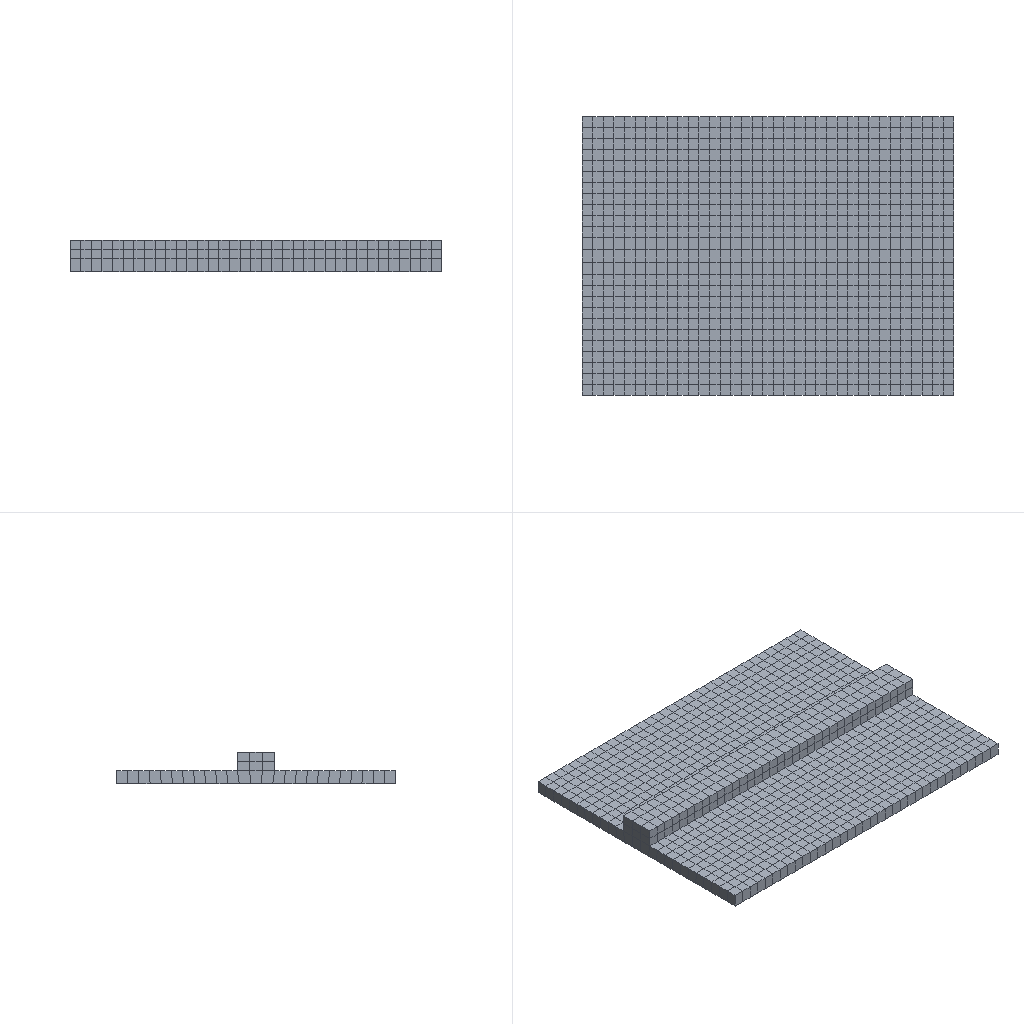Simulation study | abaqus
Set-up summary:
category,name,step,type,value,unit,region
solver,abaqus
solver,version,,,Abaqus/Standard 3DEXPERIENCE R2017x
solver,version,,,Abaqus/Standard 3DEXPERIENCE R2017x
units,not stated in the deck,,not stated
analysis,deck1,,static,coupled temperature-displacement; static
load_step,Step-del-all,Step-del-all,static,nlgeom=True
load_step,Step-add-1,Step-add-1,coupled temperature-displacement,nlgeom=True
load_step,Step-add-2,Step-add-2,coupled temperature-displacement,nlgeom=True
load_step,Step-add-3,Step-add-3,coupled temperature-displacement,nlgeom=True
load_step,Step-add-4,Step-add-4,coupled temperature-displacement,nlgeom=True
load_step,Step-add-5,Step-add-5,coupled temperature-displacement,nlgeom=True
load_step,Step-stop,Step-stop,coupled temperature-displacement,nlgeom=True
load_step,Step-add-6,Step-add-6,coupled temperature-displacement,nlgeom=True
load_step,Step-add-7,Step-add-7,coupled temperature-displacement,nlgeom=True
load_step,Step-add-8,Step-add-8,coupled temperature-displacement,nlgeom=True
load_step,Step-add-9,Step-add-9,coupled temperature-displacement,nlgeom=True
load_step,Step-add-10,Step-add-10,coupled temperature-displacement,nlgeom=True
load_step,Step-stop2,Step-stop2,coupled temperature-displacement,nlgeom=True
contact,interactions,,,general=0 pairs=0 ties=0
load_step,requested,,,13
mesh,nodes,,,2160
mesh,elements,,,1085
element_type,C3D8T,,solid,1085
load,load commands in deck,,count,1
bc,support commands in deck,,count,1
analysis,deck2,,static,coupled temperature-displacement; static
load_step,Step-del-all,Step-del-all,static,nlgeom=True
load_step,Step-add-1,Step-add-1,coupled temperature-displacement,nlgeom=True
load_step,Step-add-2,Step-add-2,coupled temperature-displacement,nlgeom=True
load_step,Step-add-3,Step-add-3,coupled temperature-displacement,nlgeom=True
load_step,Step-add-4,Step-add-4,coupled temperature-displacement,nlgeom=True
load_step,Step-add-5,Step-add-5,coupled temperature-displacement,nlgeom=True
load_step,Step-stop,Step-stop,coupled temperature-displacement,nlgeom=True
load_step,Step-add-6,Step-add-6,coupled temperature-displacement,nlgeom=True
load_step,Step-add-7,Step-add-7,coupled temperature-displacement,nlgeom=True
load_step,Step-add-8,Step-add-8,coupled temperature-displacement,nlgeom=True
load_step,Step-add-9,Step-add-9,coupled temperature-displacement,nlgeom=True
load_step,Step-add-10,Step-add-10,coupled temperature-displacement,nlgeom=True
load_step,Step-stop2,Step-stop2,coupled temperature-displacement,nlgeom=True
contact,interactions,,,general=0 pairs=0 ties=0
load_step,requested,,,13
mesh,nodes,,,2160
mesh,elements,,,1085
element_type,C3D8T,,solid,1085
load,load commands in deck,,count,1
bc,support commands in deck,,count,1
material,INCONEL,,in results
material,STEEL,,in results
material,INCONEL,,in results
material,STEEL,,in results
check,setup vs results,,match,"per instance, exact: element labels, types and connectivity; labels of the nodes the elements use; coordinates of those nodes at SINGLE_PRECISION in 1 of 1 instance(s)"
check,setup vs results,,match,"per instance, exact: element labels, types and connectivity; labels of the nodes the elements use; coordinates of those nodes at SINGLE_PRECISION in 1 of 1 instance(s)"
Results summary:
result,step,,completed,increments=1 time=0.0001/0.0001
result,step,,partial,increments=6 time=1/1.0
result,step,,partial,increments=6 time=1/1.0
result,step,,partial,increments=6 time=1/1.0
result,step,,partial,increments=6 time=1/1.0
result,step,,partial,increments=6 time=1/1.0
result,step,,completed,increments=9 time=30.0/30.0
result,step,,partial,increments=6 time=1/1.0
result,step,,partial,increments=6 time=1/1.0
result,step,,partial,increments=6 time=1/1.0
result,step,,partial,increments=6 time=1/1.0
result,step,,partial,increments=6 time=1/1.0
result,step,,completed,increments=9 time=30.0/30.0
result,analysis,,,"coupled temperature-displacement, steady state"
result,last_loadstep,,,13
result,analysis steps,,count,13
result,primary field,,,"U, NT11"
result,reaction total,,FX,0.000124,model units
result,reaction total,,FY,-3.4e-05,model units
result,reaction total,,FZ,0.000168,model units
result,step,,completed,increments=1 time=0.0001/0.0001
result,step,,partial,increments=6 time=1/1.0
result,step,,partial,increments=6 time=1/1.0
result,step,,partial,increments=6 time=1/1.0
result,step,,partial,increments=6 time=1/1.0
result,step,,partial,increments=6 time=1/1.0
result,step,,completed,increments=9 time=30.0/30.0
result,step,,partial,increments=6 time=1/1.0
result,step,,partial,increments=6 time=1/1.0
result,step,,completed,increments=6 time=1.0/1.0
result,step,,completed,increments=6 time=1.0/1.0
result,step,,completed,increments=6 time=1.0/1.0
result,step,,completed,increments=9 time=30.0/30.0
result,analysis,,,"coupled temperature-displacement, steady state"
result,last_loadstep,,,13
result,analysis steps,,count,13
result,primary field,,,"U, NT11"
result,reaction total,,FX,0.000236,model units
result,reaction total,,FY,-0.000473,model units
result,reaction total,,FZ,-0.01237,model units